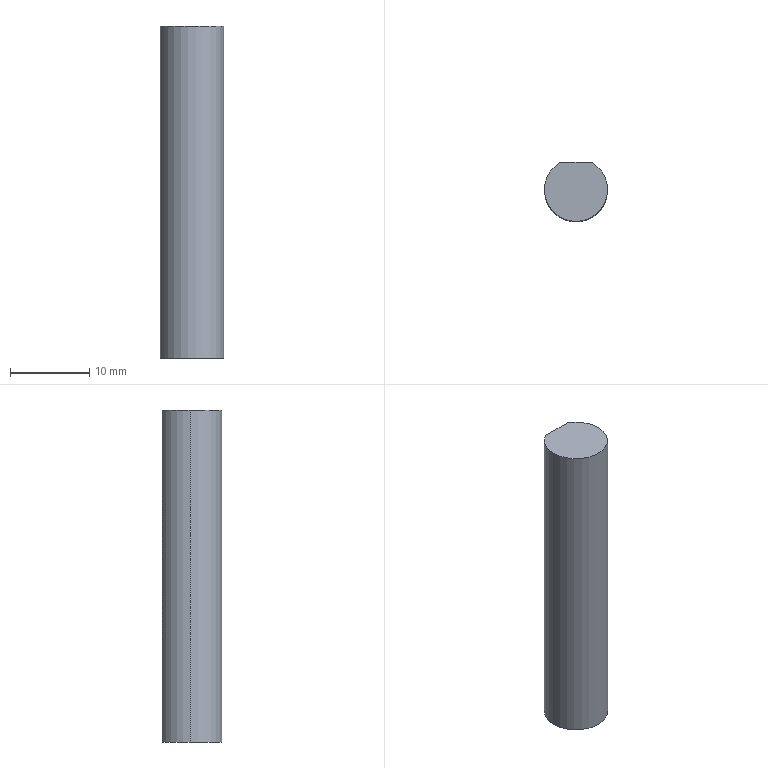Part | NX | features BREP 1 | 1 solid | 6 faces | box 8 x 7.5 x 42 mm | volume 2056 mm3 | cylinder 3 | plane 3 | commonest cylinder face diameters 8 x3
STEP:
#1=CARTESIAN_POINT('',(1.936,3.5,42.));
#2=VERTEX_POINT('',#1);
#3=CARTESIAN_POINT('',(4.,0.,42.));
#4=VERTEX_POINT('',#3);
#5=CARTESIAN_POINT('',(0.,0.,42.));
#6=DIRECTION('',(0.,0.,-1.));
#7=DIRECTION('',(-1.,0.,0.));
#8=AXIS2_PLACEMENT_3D('',#5,#6,#7);
#9=CIRCLE('',#8,4.);
#10=EDGE_CURVE('',#2,#4,#9,.T.);
#11=ORIENTED_EDGE('',*,*,#10,.T.);
#12=CARTESIAN_POINT('',(4.,0.,0.));
#13=VERTEX_POINT('',#12);
#14=CARTESIAN_POINT('',(4.,0.,42.));
#15=DIRECTION('',(0.,0.,-1.));
#16=VECTOR('',#15,1000.);
#17=LINE('',#14,#16);
#18=EDGE_CURVE('',#4,#13,#17,.T.);
#19=ORIENTED_EDGE('',*,*,#18,.T.);
#20=CARTESIAN_POINT('',(1.936,3.5,0.));
#21=VERTEX_POINT('',#20);
#22=CARTESIAN_POINT('',(0.,0.,0.));
#23=DIRECTION('',(0.,0.,1.));
#24=DIRECTION('',(-1.,0.,0.));
#25=AXIS2_PLACEMENT_3D('',#22,#23,#24);
#26=CIRCLE('',#25,4.);
#27=EDGE_CURVE('',#13,#21,#26,.T.);
#28=ORIENTED_EDGE('',*,*,#27,.T.);
#29=CARTESIAN_POINT('',(1.936,3.5,42.));
#30=DIRECTION('',(0.,0.,1.));
#31=VECTOR('',#30,1000.);
#32=LINE('',#29,#31);
#33=EDGE_CURVE('',#21,#2,#32,.T.);
#34=ORIENTED_EDGE('',*,*,#33,.T.);
#35=EDGE_LOOP('',(#11,#19,#28,#34));
#36=FACE_BOUND('',#35,.T.);
#37=CARTESIAN_POINT('',(0.,0.,42.));
#38=DIRECTION('',(0.,0.,-1.));
#39=DIRECTION('',(-1.,0.,0.));
#40=AXIS2_PLACEMENT_3D('',#37,#38,#39);
#41=CYLINDRICAL_SURFACE('',#40,4.);
#42=ADVANCED_FACE('',(#36),#41,.T.);
#43=ORIENTED_EDGE('',*,*,#18,.F.);
#44=CARTESIAN_POINT('',(-4.,0.,42.));
#45=VERTEX_POINT('',#44);
#46=CARTESIAN_POINT('',(0.,0.,42.));
#47=DIRECTION('',(0.,0.,-1.));
#48=DIRECTION('',(-1.,0.,0.));
#49=AXIS2_PLACEMENT_3D('',#46,#47,#48);
#50=CIRCLE('',#49,4.);
#51=EDGE_CURVE('',#4,#45,#50,.T.);
#52=ORIENTED_EDGE('',*,*,#51,.T.);
#53=CARTESIAN_POINT('',(-4.,0.,0.));
#54=VERTEX_POINT('',#53);
#55=CARTESIAN_POINT('',(-4.,0.,42.));
#56=DIRECTION('',(0.,0.,-1.));
#57=VECTOR('',#56,1000.);
#58=LINE('',#55,#57);
#59=EDGE_CURVE('',#45,#54,#58,.T.);
#60=ORIENTED_EDGE('',*,*,#59,.T.);
#61=CARTESIAN_POINT('',(0.,0.,0.));
#62=DIRECTION('',(0.,0.,1.));
#63=DIRECTION('',(-1.,0.,0.));
#64=AXIS2_PLACEMENT_3D('',#61,#62,#63);
#65=CIRCLE('',#64,4.);
#66=EDGE_CURVE('',#54,#13,#65,.T.);
#67=ORIENTED_EDGE('',*,*,#66,.T.);
#68=EDGE_LOOP('',(#43,#52,#60,#67));
#69=FACE_BOUND('',#68,.T.);
#70=CARTESIAN_POINT('',(0.,0.,42.));
#71=DIRECTION('',(0.,0.,-1.));
#72=DIRECTION('',(-1.,0.,0.));
#73=AXIS2_PLACEMENT_3D('',#70,#71,#72);
#74=CYLINDRICAL_SURFACE('',#73,4.);
#75=ADVANCED_FACE('',(#69),#74,.T.);
#76=ORIENTED_EDGE('',*,*,#59,.F.);
#77=CARTESIAN_POINT('',(-1.936,3.5,42.));
#78=VERTEX_POINT('',#77);
#79=CARTESIAN_POINT('',(0.,0.,42.));
#80=DIRECTION('',(0.,0.,-1.));
#81=DIRECTION('',(-1.,0.,0.));
#82=AXIS2_PLACEMENT_3D('',#79,#80,#81);
#83=CIRCLE('',#82,4.);
#84=EDGE_CURVE('',#45,#78,#83,.T.);
#85=ORIENTED_EDGE('',*,*,#84,.T.);
#86=CARTESIAN_POINT('',(-1.936,3.5,0.));
#87=VERTEX_POINT('',#86);
#88=CARTESIAN_POINT('',(-1.936,3.5,42.));
#89=DIRECTION('',(0.,0.,-1.));
#90=VECTOR('',#89,1000.);
#91=LINE('',#88,#90);
#92=EDGE_CURVE('',#78,#87,#91,.T.);
#93=ORIENTED_EDGE('',*,*,#92,.T.);
#94=CARTESIAN_POINT('',(0.,0.,0.));
#95=DIRECTION('',(0.,0.,1.));
#96=DIRECTION('',(-1.,0.,0.));
#97=AXIS2_PLACEMENT_3D('',#94,#95,#96);
#98=CIRCLE('',#97,4.);
#99=EDGE_CURVE('',#87,#54,#98,.T.);
#100=ORIENTED_EDGE('',*,*,#99,.T.);
#101=EDGE_LOOP('',(#76,#85,#93,#100));
#102=FACE_BOUND('',#101,.T.);
#103=CARTESIAN_POINT('',(0.,0.,42.));
#104=DIRECTION('',(0.,0.,-1.));
#105=DIRECTION('',(-1.,0.,0.));
#106=AXIS2_PLACEMENT_3D('',#103,#104,#105);
#107=CYLINDRICAL_SURFACE('',#106,4.);
#108=ADVANCED_FACE('',(#102),#107,.T.);
#109=CARTESIAN_POINT('',(0.,3.5,0.));
#110=DIRECTION('',(-1.,0.,0.));
#111=VECTOR('',#110,1000.);
#112=LINE('',#109,#111);
#113=EDGE_CURVE('',#21,#87,#112,.T.);
#114=ORIENTED_EDGE('',*,*,#113,.F.);
#115=ORIENTED_EDGE('',*,*,#27,.F.);
#116=ORIENTED_EDGE('',*,*,#66,.F.);
#117=ORIENTED_EDGE('',*,*,#99,.F.);
#118=EDGE_LOOP('',(#114,#115,#116,#117));
#119=FACE_BOUND('',#118,.T.);
#120=CARTESIAN_POINT('',(0.,0.,0.));
#121=DIRECTION('',(0.,0.,1.));
#122=DIRECTION('',(1.,0.,0.));
#123=AXIS2_PLACEMENT_3D('',#120,#121,#122);
#124=PLANE('',#123);
#125=ADVANCED_FACE('',(#119),#124,.F.);
#126=ORIENTED_EDGE('',*,*,#10,.F.);
#127=CARTESIAN_POINT('',(0.,3.5,42.));
#128=DIRECTION('',(-1.,0.,0.));
#129=VECTOR('',#128,1000.);
#130=LINE('',#127,#129);
#131=EDGE_CURVE('',#2,#78,#130,.T.);
#132=ORIENTED_EDGE('',*,*,#131,.T.);
#133=ORIENTED_EDGE('',*,*,#84,.F.);
#134=ORIENTED_EDGE('',*,*,#51,.F.);
#135=EDGE_LOOP('',(#126,#132,#133,#134));
#136=FACE_BOUND('',#135,.T.);
#137=CARTESIAN_POINT('',(0.,0.,42.));
#138=DIRECTION('',(0.,0.,1.));
#139=DIRECTION('',(1.,0.,0.));
#140=AXIS2_PLACEMENT_3D('',#137,#138,#139);
#141=PLANE('',#140);
#142=ADVANCED_FACE('',(#136),#141,.T.);
#143=ORIENTED_EDGE('',*,*,#33,.F.);
#144=ORIENTED_EDGE('',*,*,#113,.T.);
#145=ORIENTED_EDGE('',*,*,#92,.F.);
#146=ORIENTED_EDGE('',*,*,#131,.F.);
#147=EDGE_LOOP('',(#143,#144,#145,#146));
#148=FACE_BOUND('',#147,.T.);
#149=CARTESIAN_POINT('',(-6.733,3.5,-8.));
#150=DIRECTION('',(0.,-1.,0.));
#151=DIRECTION('',(0.,0.,-1.));
#152=AXIS2_PLACEMENT_3D('',#149,#150,#151);
#153=PLANE('',#152);
#154=ADVANCED_FACE('',(#148),#153,.F.);
#155=CLOSED_SHELL('',(#42,#75,#108,#125,#142,#154));
#156=MANIFOLD_SOLID_BREP('',#155);
#157=(LENGTH_UNIT()NAMED_UNIT(*)SI_UNIT(.MILLI.,.METRE.));
#158=UNCERTAINTY_MEASURE_WITH_UNIT(LENGTH_MEASURE(0.00001),#157,'','');
#159=(NAMED_UNIT(*)PLANE_ANGLE_UNIT()SI_UNIT($,.RADIAN.));
#160=(NAMED_UNIT(*)SI_UNIT($,.STERADIAN.)SOLID_ANGLE_UNIT());
#161=(GEOMETRIC_REPRESENTATION_CONTEXT(3)GLOBAL_UNCERTAINTY_ASSIGNED_CONTEXT((#158))GLOBAL_UNIT_ASSIGNED_CONTEXT((#157,#159,#160))REPRESENTATION_CONTEXT('',''));
#162=ADVANCED_BREP_SHAPE_REPRESENTATION('',(#156),#161);